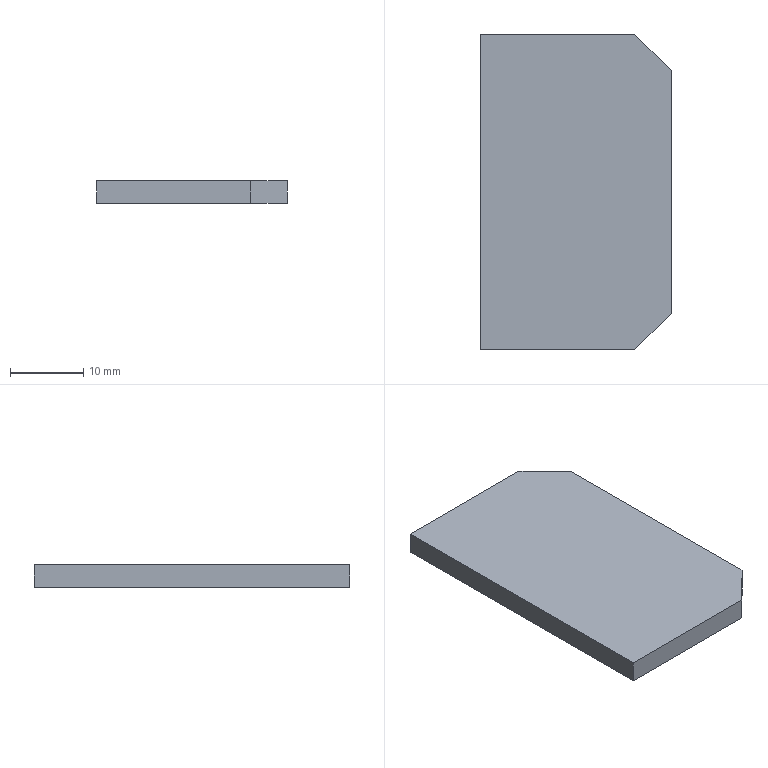Part | SolidWorks | features Chamfer 1, Extrusion 1 | 1 solid | 8 faces | box 26 x 43 x 3 mm | volume 3279 mm3 | plane 8
STEP:
#1=CARTESIAN_POINT('',(0.,43.,0.));
#2=VERTEX_POINT('',#1);
#3=CARTESIAN_POINT('',(0.,0.,0.));
#4=VERTEX_POINT('',#3);
#5=CARTESIAN_POINT('',(0.,43.,0.));
#6=DIRECTION('',(0.,-1.,0.));
#7=VECTOR('',#6,1000.);
#8=LINE('',#5,#7);
#9=EDGE_CURVE('',#2,#4,#8,.T.);
#10=ORIENTED_EDGE('',*,*,#9,.T.);
#11=CARTESIAN_POINT('',(0.,0.,3.));
#12=VERTEX_POINT('',#11);
#13=CARTESIAN_POINT('',(0.,0.,3.));
#14=DIRECTION('',(0.,0.,-1.));
#15=VECTOR('',#14,1000.);
#16=LINE('',#13,#15);
#17=EDGE_CURVE('',#12,#4,#16,.T.);
#18=ORIENTED_EDGE('',*,*,#17,.F.);
#19=CARTESIAN_POINT('',(0.,43.,3.));
#20=VERTEX_POINT('',#19);
#21=CARTESIAN_POINT('',(0.,43.,3.));
#22=DIRECTION('',(0.,-1.,0.));
#23=VECTOR('',#22,1000.);
#24=LINE('',#21,#23);
#25=EDGE_CURVE('',#20,#12,#24,.T.);
#26=ORIENTED_EDGE('',*,*,#25,.F.);
#27=CARTESIAN_POINT('',(0.,43.,3.));
#28=DIRECTION('',(0.,0.,-1.));
#29=VECTOR('',#28,1000.);
#30=LINE('',#27,#29);
#31=EDGE_CURVE('',#20,#2,#30,.T.);
#32=ORIENTED_EDGE('',*,*,#31,.T.);
#33=EDGE_LOOP('',(#10,#18,#26,#32));
#34=FACE_OUTER_BOUND('',#33,.T.);
#35=CARTESIAN_POINT('',(0.,43.,3.));
#36=DIRECTION('',(1.,0.,0.));
#37=DIRECTION('',(0.,1.,0.));
#38=AXIS2_PLACEMENT_3D('',#35,#36,#37);
#39=PLANE('',#38);
#40=ADVANCED_FACE('',(#34),#39,.F.);
#41=CARTESIAN_POINT('',(21.,0.,0.));
#42=VERTEX_POINT('',#41);
#43=CARTESIAN_POINT('',(0.,0.,0.));
#44=DIRECTION('',(1.,0.,0.));
#45=VECTOR('',#44,1000.);
#46=LINE('',#43,#45);
#47=EDGE_CURVE('',#4,#42,#46,.T.);
#48=ORIENTED_EDGE('',*,*,#47,.T.);
#49=CARTESIAN_POINT('',(21.,0.,3.));
#50=VERTEX_POINT('',#49);
#51=CARTESIAN_POINT('',(21.,0.,3.));
#52=DIRECTION('',(0.,0.,1.));
#53=VECTOR('',#52,1000.);
#54=LINE('',#51,#53);
#55=EDGE_CURVE('',#42,#50,#54,.T.);
#56=ORIENTED_EDGE('',*,*,#55,.T.);
#57=CARTESIAN_POINT('',(0.,0.,3.));
#58=DIRECTION('',(1.,0.,0.));
#59=VECTOR('',#58,1000.);
#60=LINE('',#57,#59);
#61=EDGE_CURVE('',#12,#50,#60,.T.);
#62=ORIENTED_EDGE('',*,*,#61,.F.);
#63=ORIENTED_EDGE('',*,*,#17,.T.);
#64=EDGE_LOOP('',(#48,#56,#62,#63));
#65=FACE_OUTER_BOUND('',#64,.T.);
#66=CARTESIAN_POINT('',(0.,0.,3.));
#67=DIRECTION('',(0.,1.,0.));
#68=DIRECTION('',(0.,0.,1.));
#69=AXIS2_PLACEMENT_3D('',#66,#67,#68);
#70=PLANE('',#69);
#71=ADVANCED_FACE('',(#65),#70,.F.);
#72=CARTESIAN_POINT('',(26.,5.,3.));
#73=VERTEX_POINT('',#72);
#74=CARTESIAN_POINT('',(26.,38.,3.));
#75=VERTEX_POINT('',#74);
#76=CARTESIAN_POINT('',(26.,0.,3.));
#77=DIRECTION('',(0.,1.,0.));
#78=VECTOR('',#77,1000.);
#79=LINE('',#76,#78);
#80=EDGE_CURVE('',#73,#75,#79,.T.);
#81=ORIENTED_EDGE('',*,*,#80,.F.);
#82=CARTESIAN_POINT('',(26.,5.,0.));
#83=VERTEX_POINT('',#82);
#84=CARTESIAN_POINT('',(26.,5.,3.));
#85=DIRECTION('',(0.,0.,-1.));
#86=VECTOR('',#85,1000.);
#87=LINE('',#84,#86);
#88=EDGE_CURVE('',#73,#83,#87,.T.);
#89=ORIENTED_EDGE('',*,*,#88,.T.);
#90=CARTESIAN_POINT('',(26.,38.,0.));
#91=VERTEX_POINT('',#90);
#92=CARTESIAN_POINT('',(26.,0.,0.));
#93=DIRECTION('',(0.,1.,0.));
#94=VECTOR('',#93,1000.);
#95=LINE('',#92,#94);
#96=EDGE_CURVE('',#83,#91,#95,.T.);
#97=ORIENTED_EDGE('',*,*,#96,.T.);
#98=CARTESIAN_POINT('',(26.,38.,3.));
#99=DIRECTION('',(0.,0.,1.));
#100=VECTOR('',#99,1000.);
#101=LINE('',#98,#100);
#102=EDGE_CURVE('',#91,#75,#101,.T.);
#103=ORIENTED_EDGE('',*,*,#102,.T.);
#104=EDGE_LOOP('',(#81,#89,#97,#103));
#105=FACE_OUTER_BOUND('',#104,.T.);
#106=CARTESIAN_POINT('',(26.,0.,3.));
#107=DIRECTION('',(-1.,0.,0.));
#108=DIRECTION('',(0.,-1.,0.));
#109=AXIS2_PLACEMENT_3D('',#106,#107,#108);
#110=PLANE('',#109);
#111=ADVANCED_FACE('',(#105),#110,.F.);
#112=CARTESIAN_POINT('',(21.,43.,3.));
#113=VERTEX_POINT('',#112);
#114=CARTESIAN_POINT('',(26.,43.,3.));
#115=DIRECTION('',(-1.,0.,0.));
#116=VECTOR('',#115,1000.);
#117=LINE('',#114,#116);
#118=EDGE_CURVE('',#113,#20,#117,.T.);
#119=ORIENTED_EDGE('',*,*,#118,.F.);
#120=CARTESIAN_POINT('',(21.,43.,0.));
#121=VERTEX_POINT('',#120);
#122=CARTESIAN_POINT('',(21.,43.,3.));
#123=DIRECTION('',(0.,0.,-1.));
#124=VECTOR('',#123,1000.);
#125=LINE('',#122,#124);
#126=EDGE_CURVE('',#113,#121,#125,.T.);
#127=ORIENTED_EDGE('',*,*,#126,.T.);
#128=CARTESIAN_POINT('',(26.,43.,0.));
#129=DIRECTION('',(-1.,0.,0.));
#130=VECTOR('',#129,1000.);
#131=LINE('',#128,#130);
#132=EDGE_CURVE('',#121,#2,#131,.T.);
#133=ORIENTED_EDGE('',*,*,#132,.T.);
#134=ORIENTED_EDGE('',*,*,#31,.F.);
#135=EDGE_LOOP('',(#119,#127,#133,#134));
#136=FACE_OUTER_BOUND('',#135,.T.);
#137=CARTESIAN_POINT('',(26.,43.,3.));
#138=DIRECTION('',(0.,-1.,0.));
#139=DIRECTION('',(1.,0.,0.));
#140=AXIS2_PLACEMENT_3D('',#137,#138,#139);
#141=PLANE('',#140);
#142=ADVANCED_FACE('',(#136),#141,.F.);
#143=ORIENTED_EDGE('',*,*,#61,.T.);
#144=CARTESIAN_POINT('',(10.5,-10.5,3.));
#145=DIRECTION('',(0.7071,0.7071,0.));
#146=VECTOR('',#145,1000.);
#147=LINE('',#144,#146);
#148=EDGE_CURVE('',#50,#73,#147,.T.);
#149=ORIENTED_EDGE('',*,*,#148,.T.);
#150=ORIENTED_EDGE('',*,*,#80,.T.);
#151=CARTESIAN_POINT('',(32.,32.,3.));
#152=DIRECTION('',(-0.7071,0.7071,0.));
#153=VECTOR('',#152,1000.);
#154=LINE('',#151,#153);
#155=EDGE_CURVE('',#75,#113,#154,.T.);
#156=ORIENTED_EDGE('',*,*,#155,.T.);
#157=ORIENTED_EDGE('',*,*,#118,.T.);
#158=ORIENTED_EDGE('',*,*,#25,.T.);
#159=EDGE_LOOP('',(#143,#149,#150,#156,#157,#158));
#160=FACE_OUTER_BOUND('',#159,.T.);
#161=CARTESIAN_POINT('',(0.,0.,3.));
#162=DIRECTION('',(0.,0.,1.));
#163=DIRECTION('',(1.,0.,0.));
#164=AXIS2_PLACEMENT_3D('',#161,#162,#163);
#165=PLANE('',#164);
#166=ADVANCED_FACE('',(#160),#165,.T.);
#167=ORIENTED_EDGE('',*,*,#96,.F.);
#168=CARTESIAN_POINT('',(26.,5.,0.));
#169=DIRECTION('',(-0.7071,-0.7071,0.));
#170=VECTOR('',#169,1000.);
#171=LINE('',#168,#170);
#172=EDGE_CURVE('',#83,#42,#171,.T.);
#173=ORIENTED_EDGE('',*,*,#172,.T.);
#174=ORIENTED_EDGE('',*,*,#47,.F.);
#175=ORIENTED_EDGE('',*,*,#9,.F.);
#176=ORIENTED_EDGE('',*,*,#132,.F.);
#177=CARTESIAN_POINT('',(21.,43.,0.));
#178=DIRECTION('',(0.7071,-0.7071,0.));
#179=VECTOR('',#178,1000.);
#180=LINE('',#177,#179);
#181=EDGE_CURVE('',#121,#91,#180,.T.);
#182=ORIENTED_EDGE('',*,*,#181,.T.);
#183=EDGE_LOOP('',(#167,#173,#174,#175,#176,#182));
#184=FACE_OUTER_BOUND('',#183,.T.);
#185=CARTESIAN_POINT('',(0.,0.,0.));
#186=DIRECTION('',(0.,0.,1.));
#187=DIRECTION('',(1.,0.,0.));
#188=AXIS2_PLACEMENT_3D('',#185,#186,#187);
#189=PLANE('',#188);
#190=ADVANCED_FACE('',(#184),#189,.F.);
#191=ORIENTED_EDGE('',*,*,#148,.F.);
#192=ORIENTED_EDGE('',*,*,#55,.F.);
#193=ORIENTED_EDGE('',*,*,#172,.F.);
#194=ORIENTED_EDGE('',*,*,#88,.F.);
#195=EDGE_LOOP('',(#191,#192,#193,#194));
#196=FACE_OUTER_BOUND('',#195,.T.);
#197=CARTESIAN_POINT('',(26.,5.,3.));
#198=DIRECTION('',(-0.7071,0.7071,0.));
#199=DIRECTION('',(0.,0.,-1.));
#200=AXIS2_PLACEMENT_3D('',#197,#198,#199);
#201=PLANE('',#200);
#202=ADVANCED_FACE('',(#196),#201,.F.);
#203=ORIENTED_EDGE('',*,*,#155,.F.);
#204=ORIENTED_EDGE('',*,*,#102,.F.);
#205=ORIENTED_EDGE('',*,*,#181,.F.);
#206=ORIENTED_EDGE('',*,*,#126,.F.);
#207=EDGE_LOOP('',(#203,#204,#205,#206));
#208=FACE_OUTER_BOUND('',#207,.T.);
#209=CARTESIAN_POINT('',(21.,43.,3.));
#210=DIRECTION('',(-0.7071,-0.7071,0.));
#211=DIRECTION('',(0.,0.,-1.));
#212=AXIS2_PLACEMENT_3D('',#209,#210,#211);
#213=PLANE('',#212);
#214=ADVANCED_FACE('',(#208),#213,.F.);
#215=CLOSED_SHELL('',(#40,#71,#111,#142,#166,#190,#202,#214));
#216=MANIFOLD_SOLID_BREP('',#215);
#217=CARTESIAN_POINT('',(0.,0.,0.));
#218=DIRECTION('',(0.,0.,1.));
#219=DIRECTION('',(1.,0.,0.));
#220=AXIS2_PLACEMENT_3D('',#217,#218,#219);
#221=(LENGTH_UNIT()NAMED_UNIT(*)SI_UNIT(.MILLI.,.METRE.));
#222=UNCERTAINTY_MEASURE_WITH_UNIT(LENGTH_MEASURE(0.00001),#221,'','');
#223=(NAMED_UNIT(*)PLANE_ANGLE_UNIT()SI_UNIT($,.RADIAN.));
#224=(NAMED_UNIT(*)SI_UNIT($,.STERADIAN.)SOLID_ANGLE_UNIT());
#225=(GEOMETRIC_REPRESENTATION_CONTEXT(3)GLOBAL_UNCERTAINTY_ASSIGNED_CONTEXT((#222))GLOBAL_UNIT_ASSIGNED_CONTEXT((#221,#223,#224))REPRESENTATION_CONTEXT('',''));
#226=ADVANCED_BREP_SHAPE_REPRESENTATION('',(#216,#220),#225);